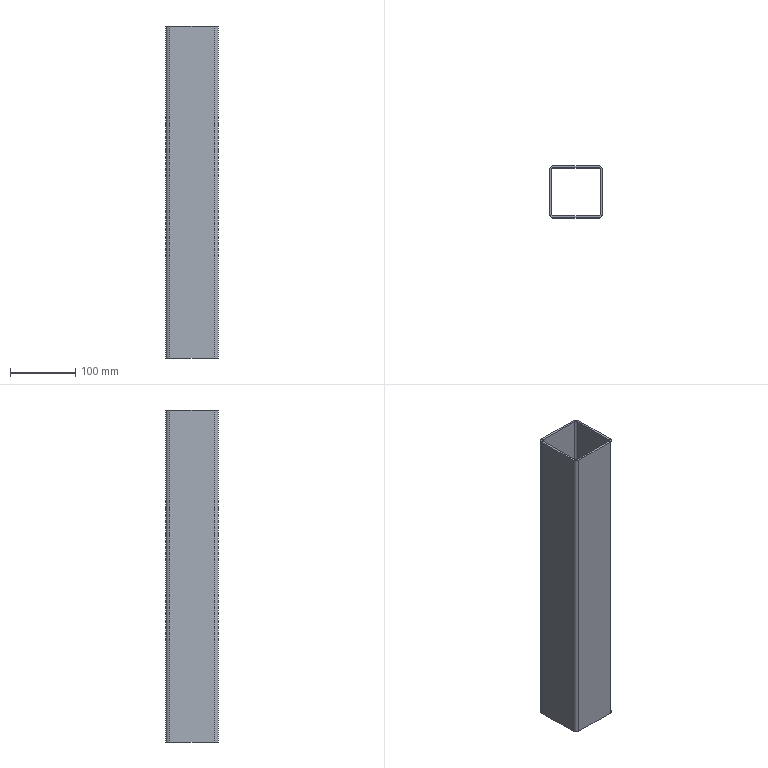Part | STEP file | Copy (1) of SN10_008_006-01_TUBO_QUADRADO | 1 solid | 18 faces | box 80 x 80 x 507.179 mm | volume 456879 mm3 | plane 10 | cylinder 8 | commonest cylinder face diameters 6 x4 12 x4
STEP:
#1=CARTESIAN_POINT('',(0.,0.,0.));
#2=DIRECTION('',(0.,0.,1.));
#3=DIRECTION('',(1.,0.,0.));
#4=AXIS2_PLACEMENT_3D('',#1,#2,#3);
#5=CARTESIAN_POINT('',(323.629,344.,-61.18));
#6=VERTEX_POINT('',#5);
#7=CARTESIAN_POINT('',(317.629,350.,-61.18));
#8=VERTEX_POINT('',#7);
#9=CARTESIAN_POINT('',(317.629,344.,-61.18));
#10=DIRECTION('',(0.,0.,1.));
#11=DIRECTION('',(1.,0.,0.));
#12=AXIS2_PLACEMENT_3D('',#9,#10,#11);
#13=CIRCLE('',#12,6.);
#14=CARTESIAN_POINT('',(361.047,350.,-61.18));
#15=DIRECTION('',(0.,0.,1.));
#16=DIRECTION('',(1.,0.,0.));
#17=AXIS2_PLACEMENT_3D('',#14,#15,#16);
#18=PLANE('',#17);
#19=CARTESIAN_POINT('',(-43.418,-6.));
#20=DIRECTION('',(1.,0.));
#21=AXIS2_PLACEMENT_2D('',#19,#20);
#22=CIRCLE('',#21,6.);
#23=(GEOMETRIC_REPRESENTATION_CONTEXT(2)PARAMETRIC_REPRESENTATION_CONTEXT()REPRESENTATION_CONTEXT('',''));
#24=DEFINITIONAL_REPRESENTATION('',(#22),#23);
#25=PCURVE('',#18,#24);
#26=CARTESIAN_POINT('',(317.629,344.,176.11));
#27=DIRECTION('',(0.,0.,1.));
#28=DIRECTION('',(1.,0.,0.));
#29=AXIS2_PLACEMENT_3D('',#26,#27,#28);
#30=CYLINDRICAL_SURFACE('',#29,6.);
#31=CARTESIAN_POINT('',(0.,-237.289));
#32=DIRECTION('',(1.,0.));
#33=VECTOR('',#32,1.);
#34=LINE('',#31,#33);
#35=(GEOMETRIC_REPRESENTATION_CONTEXT(2)PARAMETRIC_REPRESENTATION_CONTEXT()REPRESENTATION_CONTEXT('',''));
#36=DEFINITIONAL_REPRESENTATION('',(#34),#35);
#37=PCURVE('',#30,#36);
#38=SURFACE_CURVE('',#13,(#25,#37),.PCURVE_S1.);
#39=EDGE_CURVE('',#6,#8,#38,.T.);
#40=ORIENTED_EDGE('',*,*,#39,.F.);
#41=CARTESIAN_POINT('',(323.629,276.,-61.18));
#42=VERTEX_POINT('',#41);
#43=CARTESIAN_POINT('',(323.629,344.,-61.18));
#44=DIRECTION('',(0.,-1.,0.));
#45=VECTOR('',#44,1.);
#46=LINE('',#43,#45);
#47=CARTESIAN_POINT('',(-37.418,-6.));
#48=DIRECTION('',(0.,-1.));
#49=VECTOR('',#48,1.);
#50=LINE('',#47,#49);
#51=(GEOMETRIC_REPRESENTATION_CONTEXT(2)PARAMETRIC_REPRESENTATION_CONTEXT()REPRESENTATION_CONTEXT('',''));
#52=DEFINITIONAL_REPRESENTATION('',(#50),#51);
#53=PCURVE('',#18,#52);
#54=CARTESIAN_POINT('',(323.629,344.,-115.));
#55=DIRECTION('',(-1.,0.,0.));
#56=DIRECTION('',(0.,0.,1.));
#57=AXIS2_PLACEMENT_3D('',#54,#55,#56);
#58=PLANE('',#57);
#59=CARTESIAN_POINT('',(53.821,0.));
#60=DIRECTION('',(0.,-1.));
#61=VECTOR('',#60,1.);
#62=LINE('',#59,#61);
#63=(GEOMETRIC_REPRESENTATION_CONTEXT(2)PARAMETRIC_REPRESENTATION_CONTEXT()REPRESENTATION_CONTEXT('',''));
#64=DEFINITIONAL_REPRESENTATION('',(#62),#63);
#65=PCURVE('',#58,#64);
#66=SURFACE_CURVE('',#46,(#53,#65),.PCURVE_S1.);
#67=EDGE_CURVE('',#6,#42,#66,.T.);
#68=ORIENTED_EDGE('',*,*,#67,.T.);
#69=CARTESIAN_POINT('',(317.629,270.,-61.18));
#70=VERTEX_POINT('',#69);
#71=CARTESIAN_POINT('',(317.629,276.,-61.18));
#72=DIRECTION('',(0.,0.,1.));
#73=DIRECTION('',(1.,0.,0.));
#74=AXIS2_PLACEMENT_3D('',#71,#72,#73);
#75=CIRCLE('',#74,6.);
#76=CARTESIAN_POINT('',(-43.418,-74.));
#77=DIRECTION('',(1.,0.));
#78=AXIS2_PLACEMENT_2D('',#76,#77);
#79=CIRCLE('',#78,6.);
#80=(GEOMETRIC_REPRESENTATION_CONTEXT(2)PARAMETRIC_REPRESENTATION_CONTEXT()REPRESENTATION_CONTEXT('',''));
#81=DEFINITIONAL_REPRESENTATION('',(#79),#80);
#82=PCURVE('',#18,#81);
#83=CARTESIAN_POINT('',(317.629,276.,176.11));
#84=DIRECTION('',(0.,0.,1.));
#85=DIRECTION('',(0.,-1.,0.));
#86=AXIS2_PLACEMENT_3D('',#83,#84,#85);
#87=CYLINDRICAL_SURFACE('',#86,6.);
#88=CARTESIAN_POINT('',(-4.712,-237.289));
#89=DIRECTION('',(1.,0.));
#90=VECTOR('',#89,1.);
#91=LINE('',#88,#90);
#92=(GEOMETRIC_REPRESENTATION_CONTEXT(2)PARAMETRIC_REPRESENTATION_CONTEXT()REPRESENTATION_CONTEXT('',''));
#93=DEFINITIONAL_REPRESENTATION('',(#91),#92);
#94=PCURVE('',#87,#93);
#95=SURFACE_CURVE('',#75,(#82,#94),.PCURVE_S1.);
#96=EDGE_CURVE('',#70,#42,#95,.T.);
#97=ORIENTED_EDGE('',*,*,#96,.F.);
#98=CARTESIAN_POINT('',(249.629,270.,-61.18));
#99=VERTEX_POINT('',#98);
#100=CARTESIAN_POINT('',(317.629,270.,-61.18));
#101=DIRECTION('',(-1.,0.,0.));
#102=VECTOR('',#101,1.);
#103=LINE('',#100,#102);
#104=CARTESIAN_POINT('',(-43.418,-80.));
#105=DIRECTION('',(-1.,0.));
#106=VECTOR('',#105,1.);
#107=LINE('',#104,#106);
#108=(GEOMETRIC_REPRESENTATION_CONTEXT(2)PARAMETRIC_REPRESENTATION_CONTEXT()REPRESENTATION_CONTEXT('',''));
#109=DEFINITIONAL_REPRESENTATION('',(#107),#108);
#110=PCURVE('',#18,#109);
#111=CARTESIAN_POINT('',(317.629,270.,-115.));
#112=DIRECTION('',(0.,1.,0.));
#113=DIRECTION('',(0.,0.,1.));
#114=AXIS2_PLACEMENT_3D('',#111,#112,#113);
#115=PLANE('',#114);
#116=CARTESIAN_POINT('',(53.821,0.));
#117=DIRECTION('',(0.,-1.));
#118=VECTOR('',#117,1.);
#119=LINE('',#116,#118);
#120=(GEOMETRIC_REPRESENTATION_CONTEXT(2)PARAMETRIC_REPRESENTATION_CONTEXT()REPRESENTATION_CONTEXT('',''));
#121=DEFINITIONAL_REPRESENTATION('',(#119),#120);
#122=PCURVE('',#115,#121);
#123=SURFACE_CURVE('',#103,(#110,#122),.PCURVE_S1.);
#124=EDGE_CURVE('',#70,#99,#123,.T.);
#125=ORIENTED_EDGE('',*,*,#124,.T.);
#126=CARTESIAN_POINT('',(243.629,276.,-61.18));
#127=VERTEX_POINT('',#126);
#128=CARTESIAN_POINT('',(249.629,276.,-61.18));
#129=DIRECTION('',(0.,0.,1.));
#130=DIRECTION('',(1.,0.,0.));
#131=AXIS2_PLACEMENT_3D('',#128,#129,#130);
#132=CIRCLE('',#131,6.);
#133=CARTESIAN_POINT('',(-111.418,-74.));
#134=DIRECTION('',(1.,0.));
#135=AXIS2_PLACEMENT_2D('',#133,#134);
#136=CIRCLE('',#135,6.);
#137=(GEOMETRIC_REPRESENTATION_CONTEXT(2)PARAMETRIC_REPRESENTATION_CONTEXT()REPRESENTATION_CONTEXT('',''));
#138=DEFINITIONAL_REPRESENTATION('',(#136),#137);
#139=PCURVE('',#18,#138);
#140=CARTESIAN_POINT('',(249.629,276.,176.11));
#141=DIRECTION('',(0.,0.,1.));
#142=DIRECTION('',(-1.,0.,0.));
#143=AXIS2_PLACEMENT_3D('',#140,#141,#142);
#144=CYLINDRICAL_SURFACE('',#143,6.);
#145=CARTESIAN_POINT('',(-3.142,-237.289));
#146=DIRECTION('',(1.,0.));
#147=VECTOR('',#146,1.);
#148=LINE('',#145,#147);
#149=(GEOMETRIC_REPRESENTATION_CONTEXT(2)PARAMETRIC_REPRESENTATION_CONTEXT()REPRESENTATION_CONTEXT('',''));
#150=DEFINITIONAL_REPRESENTATION('',(#148),#149);
#151=PCURVE('',#144,#150);
#152=SURFACE_CURVE('',#132,(#139,#151),.PCURVE_S1.);
#153=EDGE_CURVE('',#127,#99,#152,.T.);
#154=ORIENTED_EDGE('',*,*,#153,.F.);
#155=CARTESIAN_POINT('',(243.629,344.,-61.18));
#156=VERTEX_POINT('',#155);
#157=CARTESIAN_POINT('',(243.629,276.,-61.18));
#158=DIRECTION('',(0.,1.,0.));
#159=VECTOR('',#158,1.);
#160=LINE('',#157,#159);
#161=CARTESIAN_POINT('',(-117.418,-74.));
#162=DIRECTION('',(0.,1.));
#163=VECTOR('',#162,1.);
#164=LINE('',#161,#163);
#165=(GEOMETRIC_REPRESENTATION_CONTEXT(2)PARAMETRIC_REPRESENTATION_CONTEXT()REPRESENTATION_CONTEXT('',''));
#166=DEFINITIONAL_REPRESENTATION('',(#164),#165);
#167=PCURVE('',#18,#166);
#168=CARTESIAN_POINT('',(243.629,276.,-115.));
#169=DIRECTION('',(1.,0.,0.));
#170=DIRECTION('',(0.,0.,-1.));
#171=AXIS2_PLACEMENT_3D('',#168,#169,#170);
#172=PLANE('',#171);
#173=CARTESIAN_POINT('',(-53.821,0.));
#174=DIRECTION('',(0.,1.));
#175=VECTOR('',#174,1.);
#176=LINE('',#173,#175);
#177=(GEOMETRIC_REPRESENTATION_CONTEXT(2)PARAMETRIC_REPRESENTATION_CONTEXT()REPRESENTATION_CONTEXT('',''));
#178=DEFINITIONAL_REPRESENTATION('',(#176),#177);
#179=PCURVE('',#172,#178);
#180=SURFACE_CURVE('',#160,(#167,#179),.PCURVE_S1.);
#181=EDGE_CURVE('',#127,#156,#180,.T.);
#182=ORIENTED_EDGE('',*,*,#181,.T.);
#183=CARTESIAN_POINT('',(249.629,350.,-61.18));
#184=VERTEX_POINT('',#183);
#185=CARTESIAN_POINT('',(249.629,344.,-61.18));
#186=DIRECTION('',(0.,0.,1.));
#187=DIRECTION('',(1.,0.,0.));
#188=AXIS2_PLACEMENT_3D('',#185,#186,#187);
#189=CIRCLE('',#188,6.);
#190=CARTESIAN_POINT('',(-111.418,-6.));
#191=DIRECTION('',(1.,0.));
#192=AXIS2_PLACEMENT_2D('',#190,#191);
#193=CIRCLE('',#192,6.);
#194=(GEOMETRIC_REPRESENTATION_CONTEXT(2)PARAMETRIC_REPRESENTATION_CONTEXT()REPRESENTATION_CONTEXT('',''));
#195=DEFINITIONAL_REPRESENTATION('',(#193),#194);
#196=PCURVE('',#18,#195);
#197=CARTESIAN_POINT('',(249.629,344.,176.11));
#198=DIRECTION('',(0.,0.,1.));
#199=DIRECTION('',(0.,1.,0.));
#200=AXIS2_PLACEMENT_3D('',#197,#198,#199);
#201=CYLINDRICAL_SURFACE('',#200,6.);
#202=CARTESIAN_POINT('',(-1.571,-237.289));
#203=DIRECTION('',(1.,0.));
#204=VECTOR('',#203,1.);
#205=LINE('',#202,#204);
#206=(GEOMETRIC_REPRESENTATION_CONTEXT(2)PARAMETRIC_REPRESENTATION_CONTEXT()REPRESENTATION_CONTEXT('',''));
#207=DEFINITIONAL_REPRESENTATION('',(#205),#206);
#208=PCURVE('',#201,#207);
#209=SURFACE_CURVE('',#189,(#196,#208),.PCURVE_S1.);
#210=EDGE_CURVE('',#184,#156,#209,.T.);
#211=ORIENTED_EDGE('',*,*,#210,.F.);
#212=CARTESIAN_POINT('',(317.629,350.,-61.18));
#213=DIRECTION('',(-1.,0.,0.));
#214=VECTOR('',#213,1.);
#215=LINE('',#212,#214);
#216=CARTESIAN_POINT('',(-43.418,0.));
#217=DIRECTION('',(-1.,0.));
#218=VECTOR('',#217,1.);
#219=LINE('',#216,#218);
#220=(GEOMETRIC_REPRESENTATION_CONTEXT(2)PARAMETRIC_REPRESENTATION_CONTEXT()REPRESENTATION_CONTEXT('',''));
#221=DEFINITIONAL_REPRESENTATION('',(#219),#220);
#222=PCURVE('',#18,#221);
#223=CARTESIAN_POINT('',(249.629,350.,-115.));
#224=DIRECTION('',(0.,-1.,0.));
#225=DIRECTION('',(0.,0.,-1.));
#226=AXIS2_PLACEMENT_3D('',#223,#224,#225);
#227=PLANE('',#226);
#228=CARTESIAN_POINT('',(-53.821,68.));
#229=DIRECTION('',(0.,-1.));
#230=VECTOR('',#229,1.);
#231=LINE('',#228,#230);
#232=(GEOMETRIC_REPRESENTATION_CONTEXT(2)PARAMETRIC_REPRESENTATION_CONTEXT()REPRESENTATION_CONTEXT('',''));
#233=DEFINITIONAL_REPRESENTATION('',(#231),#232);
#234=PCURVE('',#227,#233);
#235=SURFACE_CURVE('',#215,(#222,#234),.PCURVE_S1.);
#236=EDGE_CURVE('',#8,#184,#235,.T.);
#237=ORIENTED_EDGE('',*,*,#236,.F.);
#238=EDGE_LOOP('',(#40,#68,#97,#125,#154,#182,#211,#237));
#239=FACE_BOUND('',#238,.T.);
#240=CARTESIAN_POINT('',(249.629,347.,-61.18));
#241=VERTEX_POINT('',#240);
#242=CARTESIAN_POINT('',(246.629,344.,-61.18));
#243=VERTEX_POINT('',#242);
#244=CARTESIAN_POINT('',(249.629,344.,-61.18));
#245=DIRECTION('',(0.,0.,1.));
#246=DIRECTION('',(1.,0.,0.));
#247=AXIS2_PLACEMENT_3D('',#244,#245,#246);
#248=CIRCLE('',#247,3.);
#249=CARTESIAN_POINT('',(-111.418,-6.));
#250=DIRECTION('',(1.,0.));
#251=AXIS2_PLACEMENT_2D('',#249,#250);
#252=CIRCLE('',#251,3.);
#253=(GEOMETRIC_REPRESENTATION_CONTEXT(2)PARAMETRIC_REPRESENTATION_CONTEXT()REPRESENTATION_CONTEXT('',''));
#254=DEFINITIONAL_REPRESENTATION('',(#252),#253);
#255=PCURVE('',#18,#254);
#256=CARTESIAN_POINT('',(249.629,344.,176.11));
#257=DIRECTION('',(0.,0.,1.));
#258=DIRECTION('',(0.,1.,0.));
#259=AXIS2_PLACEMENT_3D('',#256,#257,#258);
#260=CYLINDRICAL_SURFACE('',#259,3.);
#261=CARTESIAN_POINT('',(-1.571,-237.289));
#262=DIRECTION('',(1.,0.));
#263=VECTOR('',#262,1.);
#264=LINE('',#261,#263);
#265=(GEOMETRIC_REPRESENTATION_CONTEXT(2)PARAMETRIC_REPRESENTATION_CONTEXT()REPRESENTATION_CONTEXT('',''));
#266=DEFINITIONAL_REPRESENTATION('',(#264),#265);
#267=PCURVE('',#260,#266);
#268=SURFACE_CURVE('',#248,(#255,#267),.PCURVE_S1.);
#269=EDGE_CURVE('',#241,#243,#268,.T.);
#270=ORIENTED_EDGE('',*,*,#269,.T.);
#271=CARTESIAN_POINT('',(246.629,276.,-61.18));
#272=VERTEX_POINT('',#271);
#273=CARTESIAN_POINT('',(246.629,276.,-61.18));
#274=DIRECTION('',(0.,1.,0.));
#275=VECTOR('',#274,1.);
#276=LINE('',#273,#275);
#277=CARTESIAN_POINT('',(-114.418,-74.));
#278=DIRECTION('',(0.,1.));
#279=VECTOR('',#278,1.);
#280=LINE('',#277,#279);
#281=(GEOMETRIC_REPRESENTATION_CONTEXT(2)PARAMETRIC_REPRESENTATION_CONTEXT()REPRESENTATION_CONTEXT('',''));
#282=DEFINITIONAL_REPRESENTATION('',(#280),#281);
#283=PCURVE('',#18,#282);
#284=CARTESIAN_POINT('',(246.629,276.,-115.));
#285=DIRECTION('',(1.,0.,0.));
#286=DIRECTION('',(0.,0.,-1.));
#287=AXIS2_PLACEMENT_3D('',#284,#285,#286);
#288=PLANE('',#287);
#289=CARTESIAN_POINT('',(-53.821,0.));
#290=DIRECTION('',(0.,1.));
#291=VECTOR('',#290,1.);
#292=LINE('',#289,#291);
#293=(GEOMETRIC_REPRESENTATION_CONTEXT(2)PARAMETRIC_REPRESENTATION_CONTEXT()REPRESENTATION_CONTEXT('',''));
#294=DEFINITIONAL_REPRESENTATION('',(#292),#293);
#295=PCURVE('',#288,#294);
#296=SURFACE_CURVE('',#276,(#283,#295),.PCURVE_S1.);
#297=EDGE_CURVE('',#272,#243,#296,.T.);
#298=ORIENTED_EDGE('',*,*,#297,.F.);
#299=CARTESIAN_POINT('',(249.629,273.,-61.18));
#300=VERTEX_POINT('',#299);
#301=CARTESIAN_POINT('',(249.629,276.,-61.18));
#302=DIRECTION('',(0.,0.,1.));
#303=DIRECTION('',(1.,0.,0.));
#304=AXIS2_PLACEMENT_3D('',#301,#302,#303);
#305=CIRCLE('',#304,3.);
#306=CARTESIAN_POINT('',(-111.418,-74.));
#307=DIRECTION('',(1.,0.));
#308=AXIS2_PLACEMENT_2D('',#306,#307);
#309=CIRCLE('',#308,3.);
#310=(GEOMETRIC_REPRESENTATION_CONTEXT(2)PARAMETRIC_REPRESENTATION_CONTEXT()REPRESENTATION_CONTEXT('',''));
#311=DEFINITIONAL_REPRESENTATION('',(#309),#310);
#312=PCURVE('',#18,#311);
#313=CARTESIAN_POINT('',(249.629,276.,176.11));
#314=DIRECTION('',(0.,0.,1.));
#315=DIRECTION('',(-1.,0.,0.));
#316=AXIS2_PLACEMENT_3D('',#313,#314,#315);
#317=CYLINDRICAL_SURFACE('',#316,3.);
#318=CARTESIAN_POINT('',(-3.142,-237.289));
#319=DIRECTION('',(1.,0.));
#320=VECTOR('',#319,1.);
#321=LINE('',#318,#320);
#322=(GEOMETRIC_REPRESENTATION_CONTEXT(2)PARAMETRIC_REPRESENTATION_CONTEXT()REPRESENTATION_CONTEXT('',''));
#323=DEFINITIONAL_REPRESENTATION('',(#321),#322);
#324=PCURVE('',#317,#323);
#325=SURFACE_CURVE('',#305,(#312,#324),.PCURVE_S1.);
#326=EDGE_CURVE('',#272,#300,#325,.T.);
#327=ORIENTED_EDGE('',*,*,#326,.T.);
#328=CARTESIAN_POINT('',(317.629,273.,-61.18));
#329=VERTEX_POINT('',#328);
#330=CARTESIAN_POINT('',(317.629,273.,-61.18));
#331=DIRECTION('',(-1.,0.,0.));
#332=VECTOR('',#331,1.);
#333=LINE('',#330,#332);
#334=CARTESIAN_POINT('',(-43.418,-77.));
#335=DIRECTION('',(-1.,0.));
#336=VECTOR('',#335,1.);
#337=LINE('',#334,#336);
#338=(GEOMETRIC_REPRESENTATION_CONTEXT(2)PARAMETRIC_REPRESENTATION_CONTEXT()REPRESENTATION_CONTEXT('',''));
#339=DEFINITIONAL_REPRESENTATION('',(#337),#338);
#340=PCURVE('',#18,#339);
#341=CARTESIAN_POINT('',(317.629,273.,-115.));
#342=DIRECTION('',(0.,1.,0.));
#343=DIRECTION('',(0.,0.,1.));
#344=AXIS2_PLACEMENT_3D('',#341,#342,#343);
#345=PLANE('',#344);
#346=CARTESIAN_POINT('',(53.821,0.));
#347=DIRECTION('',(0.,-1.));
#348=VECTOR('',#347,1.);
#349=LINE('',#346,#348);
#350=(GEOMETRIC_REPRESENTATION_CONTEXT(2)PARAMETRIC_REPRESENTATION_CONTEXT()REPRESENTATION_CONTEXT('',''));
#351=DEFINITIONAL_REPRESENTATION('',(#349),#350);
#352=PCURVE('',#345,#351);
#353=SURFACE_CURVE('',#333,(#340,#352),.PCURVE_S1.);
#354=EDGE_CURVE('',#329,#300,#353,.T.);
#355=ORIENTED_EDGE('',*,*,#354,.F.);
#356=CARTESIAN_POINT('',(320.629,276.,-61.18));
#357=VERTEX_POINT('',#356);
#358=CARTESIAN_POINT('',(317.629,276.,-61.18));
#359=DIRECTION('',(0.,0.,1.));
#360=DIRECTION('',(1.,0.,0.));
#361=AXIS2_PLACEMENT_3D('',#358,#359,#360);
#362=CIRCLE('',#361,3.);
#363=CARTESIAN_POINT('',(-43.418,-74.));
#364=DIRECTION('',(1.,0.));
#365=AXIS2_PLACEMENT_2D('',#363,#364);
#366=CIRCLE('',#365,3.);
#367=(GEOMETRIC_REPRESENTATION_CONTEXT(2)PARAMETRIC_REPRESENTATION_CONTEXT()REPRESENTATION_CONTEXT('',''));
#368=DEFINITIONAL_REPRESENTATION('',(#366),#367);
#369=PCURVE('',#18,#368);
#370=CARTESIAN_POINT('',(317.629,276.,176.11));
#371=DIRECTION('',(0.,0.,1.));
#372=DIRECTION('',(0.,-1.,0.));
#373=AXIS2_PLACEMENT_3D('',#370,#371,#372);
#374=CYLINDRICAL_SURFACE('',#373,3.);
#375=CARTESIAN_POINT('',(-4.712,-237.289));
#376=DIRECTION('',(1.,0.));
#377=VECTOR('',#376,1.);
#378=LINE('',#375,#377);
#379=(GEOMETRIC_REPRESENTATION_CONTEXT(2)PARAMETRIC_REPRESENTATION_CONTEXT()REPRESENTATION_CONTEXT('',''));
#380=DEFINITIONAL_REPRESENTATION('',(#378),#379);
#381=PCURVE('',#374,#380);
#382=SURFACE_CURVE('',#362,(#369,#381),.PCURVE_S1.);
#383=EDGE_CURVE('',#329,#357,#382,.T.);
#384=ORIENTED_EDGE('',*,*,#383,.T.);
#385=CARTESIAN_POINT('',(320.629,344.,-61.18));
#386=VERTEX_POINT('',#385);
#387=CARTESIAN_POINT('',(320.629,344.,-61.18));
#388=DIRECTION('',(0.,-1.,0.));
#389=VECTOR('',#388,1.);
#390=LINE('',#387,#389);
#391=CARTESIAN_POINT('',(-40.418,-6.));
#392=DIRECTION('',(0.,-1.));
#393=VECTOR('',#392,1.);
#394=LINE('',#391,#393);
#395=(GEOMETRIC_REPRESENTATION_CONTEXT(2)PARAMETRIC_REPRESENTATION_CONTEXT()REPRESENTATION_CONTEXT('',''));
#396=DEFINITIONAL_REPRESENTATION('',(#394),#395);
#397=PCURVE('',#18,#396);
#398=CARTESIAN_POINT('',(320.629,344.,-115.));
#399=DIRECTION('',(-1.,0.,0.));
#400=DIRECTION('',(0.,0.,1.));
#401=AXIS2_PLACEMENT_3D('',#398,#399,#400);
#402=PLANE('',#401);
#403=CARTESIAN_POINT('',(53.821,0.));
#404=DIRECTION('',(0.,-1.));
#405=VECTOR('',#404,1.);
#406=LINE('',#403,#405);
#407=(GEOMETRIC_REPRESENTATION_CONTEXT(2)PARAMETRIC_REPRESENTATION_CONTEXT()REPRESENTATION_CONTEXT('',''));
#408=DEFINITIONAL_REPRESENTATION('',(#406),#407);
#409=PCURVE('',#402,#408);
#410=SURFACE_CURVE('',#390,(#397,#409),.PCURVE_S1.);
#411=EDGE_CURVE('',#386,#357,#410,.T.);
#412=ORIENTED_EDGE('',*,*,#411,.F.);
#413=CARTESIAN_POINT('',(317.629,347.,-61.18));
#414=VERTEX_POINT('',#413);
#415=CARTESIAN_POINT('',(317.629,344.,-61.18));
#416=DIRECTION('',(0.,0.,1.));
#417=DIRECTION('',(1.,0.,0.));
#418=AXIS2_PLACEMENT_3D('',#415,#416,#417);
#419=CIRCLE('',#418,3.);
#420=CARTESIAN_POINT('',(-43.418,-6.));
#421=DIRECTION('',(1.,0.));
#422=AXIS2_PLACEMENT_2D('',#420,#421);
#423=CIRCLE('',#422,3.);
#424=(GEOMETRIC_REPRESENTATION_CONTEXT(2)PARAMETRIC_REPRESENTATION_CONTEXT()REPRESENTATION_CONTEXT('',''));
#425=DEFINITIONAL_REPRESENTATION('',(#423),#424);
#426=PCURVE('',#18,#425);
#427=CARTESIAN_POINT('',(317.629,344.,176.11));
#428=DIRECTION('',(0.,0.,1.));
#429=DIRECTION('',(1.,0.,0.));
#430=AXIS2_PLACEMENT_3D('',#427,#428,#429);
#431=CYLINDRICAL_SURFACE('',#430,3.);
#432=CARTESIAN_POINT('',(0.,-237.289));
#433=DIRECTION('',(1.,0.));
#434=VECTOR('',#433,1.);
#435=LINE('',#432,#434);
#436=(GEOMETRIC_REPRESENTATION_CONTEXT(2)PARAMETRIC_REPRESENTATION_CONTEXT()REPRESENTATION_CONTEXT('',''));
#437=DEFINITIONAL_REPRESENTATION('',(#435),#436);
#438=PCURVE('',#431,#437);
#439=SURFACE_CURVE('',#419,(#426,#438),.PCURVE_S1.);
#440=EDGE_CURVE('',#386,#414,#439,.T.);
#441=ORIENTED_EDGE('',*,*,#440,.T.);
#442=CARTESIAN_POINT('',(249.629,347.,-61.18));
#443=DIRECTION('',(1.,0.,0.));
#444=VECTOR('',#443,1.);
#445=LINE('',#442,#444);
#446=CARTESIAN_POINT('',(-111.418,-3.));
#447=DIRECTION('',(1.,0.));
#448=VECTOR('',#447,1.);
#449=LINE('',#446,#448);
#450=(GEOMETRIC_REPRESENTATION_CONTEXT(2)PARAMETRIC_REPRESENTATION_CONTEXT()REPRESENTATION_CONTEXT('',''));
#451=DEFINITIONAL_REPRESENTATION('',(#449),#450);
#452=PCURVE('',#18,#451);
#453=CARTESIAN_POINT('',(249.629,347.,-115.));
#454=DIRECTION('',(0.,-1.,0.));
#455=DIRECTION('',(0.,0.,-1.));
#456=AXIS2_PLACEMENT_3D('',#453,#454,#455);
#457=PLANE('',#456);
#458=CARTESIAN_POINT('',(-53.821,0.));
#459=DIRECTION('',(0.,1.));
#460=VECTOR('',#459,1.);
#461=LINE('',#458,#460);
#462=(GEOMETRIC_REPRESENTATION_CONTEXT(2)PARAMETRIC_REPRESENTATION_CONTEXT()REPRESENTATION_CONTEXT('',''));
#463=DEFINITIONAL_REPRESENTATION('',(#461),#462);
#464=PCURVE('',#457,#463);
#465=SURFACE_CURVE('',#445,(#452,#464),.PCURVE_S1.);
#466=EDGE_CURVE('',#241,#414,#465,.T.);
#467=ORIENTED_EDGE('',*,*,#466,.F.);
#468=EDGE_LOOP('',(#270,#298,#327,#355,#384,#412,#441,#467));
#469=FACE_BOUND('',#468,.T.);
#470=ADVANCED_FACE('',(#239,#469),#18,.F.);
#471=ORIENTED_EDGE('',*,*,#236,.T.);
#472=CARTESIAN_POINT('',(249.629,350.,446.));
#473=VERTEX_POINT('',#472);
#474=CARTESIAN_POINT('',(249.629,350.,446.));
#475=DIRECTION('',(0.,0.,-1.));
#476=VECTOR('',#475,1.);
#477=LINE('',#474,#476);
#478=CARTESIAN_POINT('',(-561.,0.));
#479=DIRECTION('',(1.,0.));
#480=VECTOR('',#479,1.);
#481=LINE('',#478,#480);
#482=(GEOMETRIC_REPRESENTATION_CONTEXT(2)PARAMETRIC_REPRESENTATION_CONTEXT()REPRESENTATION_CONTEXT('',''));
#483=DEFINITIONAL_REPRESENTATION('',(#481),#482);
#484=PCURVE('',#227,#483);
#485=CARTESIAN_POINT('',(0.,269.89));
#486=DIRECTION('',(0.,-1.));
#487=VECTOR('',#486,1.);
#488=LINE('',#485,#487);
#489=(GEOMETRIC_REPRESENTATION_CONTEXT(2)PARAMETRIC_REPRESENTATION_CONTEXT()REPRESENTATION_CONTEXT('',''));
#490=DEFINITIONAL_REPRESENTATION('',(#488),#489);
#491=PCURVE('',#201,#490);
#492=SURFACE_CURVE('',#477,(#484,#491),.PCURVE_S1.);
#493=EDGE_CURVE('',#473,#184,#492,.T.);
#494=ORIENTED_EDGE('',*,*,#493,.F.);
#495=CARTESIAN_POINT('',(317.629,350.,446.));
#496=VERTEX_POINT('',#495);
#497=CARTESIAN_POINT('',(249.629,350.,446.));
#498=DIRECTION('',(1.,0.,0.));
#499=VECTOR('',#498,1.);
#500=LINE('',#497,#499);
#501=CARTESIAN_POINT('',(-561.,0.));
#502=DIRECTION('',(0.,1.));
#503=VECTOR('',#502,1.);
#504=LINE('',#501,#503);
#505=(GEOMETRIC_REPRESENTATION_CONTEXT(2)PARAMETRIC_REPRESENTATION_CONTEXT()REPRESENTATION_CONTEXT('',''));
#506=DEFINITIONAL_REPRESENTATION('',(#504),#505);
#507=PCURVE('',#227,#506);
#508=CARTESIAN_POINT('',(323.629,250.,446.));
#509=DIRECTION('',(0.,0.,-1.));
#510=DIRECTION('',(-1.,0.,0.));
#511=AXIS2_PLACEMENT_3D('',#508,#509,#510);
#512=PLANE('',#511);
#513=CARTESIAN_POINT('',(74.,100.));
#514=DIRECTION('',(-1.,0.));
#515=VECTOR('',#514,1.);
#516=LINE('',#513,#515);
#517=(GEOMETRIC_REPRESENTATION_CONTEXT(2)PARAMETRIC_REPRESENTATION_CONTEXT()REPRESENTATION_CONTEXT('',''));
#518=DEFINITIONAL_REPRESENTATION('',(#516),#517);
#519=PCURVE('',#512,#518);
#520=SURFACE_CURVE('',#500,(#507,#519),.PCURVE_S1.);
#521=EDGE_CURVE('',#473,#496,#520,.T.);
#522=ORIENTED_EDGE('',*,*,#521,.T.);
#523=CARTESIAN_POINT('',(317.629,350.,446.));
#524=DIRECTION('',(0.,0.,-1.));
#525=VECTOR('',#524,1.);
#526=LINE('',#523,#525);
#527=CARTESIAN_POINT('',(-561.,68.));
#528=DIRECTION('',(1.,0.));
#529=VECTOR('',#528,1.);
#530=LINE('',#527,#529);
#531=(GEOMETRIC_REPRESENTATION_CONTEXT(2)PARAMETRIC_REPRESENTATION_CONTEXT()REPRESENTATION_CONTEXT('',''));
#532=DEFINITIONAL_REPRESENTATION('',(#530),#531);
#533=PCURVE('',#227,#532);
#534=CARTESIAN_POINT('',(1.571,269.89));
#535=DIRECTION('',(0.,-1.));
#536=VECTOR('',#535,1.);
#537=LINE('',#534,#536);
#538=(GEOMETRIC_REPRESENTATION_CONTEXT(2)PARAMETRIC_REPRESENTATION_CONTEXT()REPRESENTATION_CONTEXT('',''));
#539=DEFINITIONAL_REPRESENTATION('',(#537),#538);
#540=PCURVE('',#30,#539);
#541=SURFACE_CURVE('',#526,(#533,#540),.PCURVE_S1.);
#542=EDGE_CURVE('',#496,#8,#541,.T.);
#543=ORIENTED_EDGE('',*,*,#542,.T.);
#544=EDGE_LOOP('',(#471,#494,#522,#543));
#545=FACE_BOUND('',#544,.T.);
#546=ADVANCED_FACE('',(#545),#227,.F.);
#547=ORIENTED_EDGE('',*,*,#181,.F.);
#548=CARTESIAN_POINT('',(243.629,276.,446.));
#549=VERTEX_POINT('',#548);
#550=CARTESIAN_POINT('',(243.629,276.,446.));
#551=DIRECTION('',(0.,0.,-1.));
#552=VECTOR('',#551,1.);
#553=LINE('',#550,#552);
#554=CARTESIAN_POINT('',(-561.,0.));
#555=DIRECTION('',(1.,0.));
#556=VECTOR('',#555,1.);
#557=LINE('',#554,#556);
#558=(GEOMETRIC_REPRESENTATION_CONTEXT(2)PARAMETRIC_REPRESENTATION_CONTEXT()REPRESENTATION_CONTEXT('',''));
#559=DEFINITIONAL_REPRESENTATION('',(#557),#558);
#560=PCURVE('',#172,#559);
#561=CARTESIAN_POINT('',(0.,269.89));
#562=DIRECTION('',(0.,-1.));
#563=VECTOR('',#562,1.);
#564=LINE('',#561,#563);
#565=(GEOMETRIC_REPRESENTATION_CONTEXT(2)PARAMETRIC_REPRESENTATION_CONTEXT()REPRESENTATION_CONTEXT('',''));
#566=DEFINITIONAL_REPRESENTATION('',(#564),#565);
#567=PCURVE('',#144,#566);
#568=SURFACE_CURVE('',#553,(#560,#567),.PCURVE_S1.);
#569=EDGE_CURVE('',#549,#127,#568,.T.);
#570=ORIENTED_EDGE('',*,*,#569,.F.);
#571=CARTESIAN_POINT('',(243.629,344.,446.));
#572=VERTEX_POINT('',#571);
#573=CARTESIAN_POINT('',(243.629,276.,446.));
#574=DIRECTION('',(0.,1.,0.));
#575=VECTOR('',#574,1.);
#576=LINE('',#573,#575);
#577=CARTESIAN_POINT('',(-561.,0.));
#578=DIRECTION('',(0.,1.));
#579=VECTOR('',#578,1.);
#580=LINE('',#577,#579);
#581=(GEOMETRIC_REPRESENTATION_CONTEXT(2)PARAMETRIC_REPRESENTATION_CONTEXT()REPRESENTATION_CONTEXT('',''));
#582=DEFINITIONAL_REPRESENTATION('',(#580),#581);
#583=PCURVE('',#172,#582);
#584=CARTESIAN_POINT('',(80.,26.));
#585=DIRECTION('',(0.,1.));
#586=VECTOR('',#585,1.);
#587=LINE('',#584,#586);
#588=(GEOMETRIC_REPRESENTATION_CONTEXT(2)PARAMETRIC_REPRESENTATION_CONTEXT()REPRESENTATION_CONTEXT('',''));
#589=DEFINITIONAL_REPRESENTATION('',(#587),#588);
#590=PCURVE('',#512,#589);
#591=SURFACE_CURVE('',#576,(#583,#590),.PCURVE_S1.);
#592=EDGE_CURVE('',#549,#572,#591,.T.);
#593=ORIENTED_EDGE('',*,*,#592,.T.);
#594=CARTESIAN_POINT('',(243.629,344.,446.));
#595=DIRECTION('',(0.,0.,-1.));
#596=VECTOR('',#595,1.);
#597=LINE('',#594,#596);
#598=CARTESIAN_POINT('',(-561.,68.));
#599=DIRECTION('',(1.,0.));
#600=VECTOR('',#599,1.);
#601=LINE('',#598,#600);
#602=(GEOMETRIC_REPRESENTATION_CONTEXT(2)PARAMETRIC_REPRESENTATION_CONTEXT()REPRESENTATION_CONTEXT('',''));
#603=DEFINITIONAL_REPRESENTATION('',(#601),#602);
#604=PCURVE('',#172,#603);
#605=CARTESIAN_POINT('',(1.571,269.89));
#606=DIRECTION('',(0.,-1.));
#607=VECTOR('',#606,1.);
#608=LINE('',#605,#607);
#609=(GEOMETRIC_REPRESENTATION_CONTEXT(2)PARAMETRIC_REPRESENTATION_CONTEXT()REPRESENTATION_CONTEXT('',''));
#610=DEFINITIONAL_REPRESENTATION('',(#608),#609);
#611=PCURVE('',#201,#610);
#612=SURFACE_CURVE('',#597,(#604,#611),.PCURVE_S1.);
#613=EDGE_CURVE('',#572,#156,#612,.T.);
#614=ORIENTED_EDGE('',*,*,#613,.T.);
#615=EDGE_LOOP('',(#547,#570,#593,#614));
#616=FACE_BOUND('',#615,.T.);
#617=ADVANCED_FACE('',(#616),#172,.F.);
#618=ORIENTED_EDGE('',*,*,#124,.F.);
#619=CARTESIAN_POINT('',(317.629,270.,446.));
#620=VERTEX_POINT('',#619);
#621=CARTESIAN_POINT('',(317.629,270.,446.));
#622=DIRECTION('',(0.,0.,-1.));
#623=VECTOR('',#622,1.);
#624=LINE('',#621,#623);
#625=CARTESIAN_POINT('',(561.,0.));
#626=DIRECTION('',(-1.,0.));
#627=VECTOR('',#626,1.);
#628=LINE('',#625,#627);
#629=(GEOMETRIC_REPRESENTATION_CONTEXT(2)PARAMETRIC_REPRESENTATION_CONTEXT()REPRESENTATION_CONTEXT('',''));
#630=DEFINITIONAL_REPRESENTATION('',(#628),#629);
#631=PCURVE('',#115,#630);
#632=CARTESIAN_POINT('',(0.,269.89));
#633=DIRECTION('',(0.,-1.));
#634=VECTOR('',#633,1.);
#635=LINE('',#632,#634);
#636=(GEOMETRIC_REPRESENTATION_CONTEXT(2)PARAMETRIC_REPRESENTATION_CONTEXT()REPRESENTATION_CONTEXT('',''));
#637=DEFINITIONAL_REPRESENTATION('',(#635),#636);
#638=PCURVE('',#87,#637);
#639=SURFACE_CURVE('',#624,(#631,#638),.PCURVE_S1.);
#640=EDGE_CURVE('',#620,#70,#639,.T.);
#641=ORIENTED_EDGE('',*,*,#640,.F.);
#642=CARTESIAN_POINT('',(249.629,270.,446.));
#643=VERTEX_POINT('',#642);
#644=CARTESIAN_POINT('',(317.629,270.,446.));
#645=DIRECTION('',(-1.,0.,0.));
#646=VECTOR('',#645,1.);
#647=LINE('',#644,#646);
#648=CARTESIAN_POINT('',(561.,0.));
#649=DIRECTION('',(0.,-1.));
#650=VECTOR('',#649,1.);
#651=LINE('',#648,#650);
#652=(GEOMETRIC_REPRESENTATION_CONTEXT(2)PARAMETRIC_REPRESENTATION_CONTEXT()REPRESENTATION_CONTEXT('',''));
#653=DEFINITIONAL_REPRESENTATION('',(#651),#652);
#654=PCURVE('',#115,#653);
#655=CARTESIAN_POINT('',(6.,20.));
#656=DIRECTION('',(1.,0.));
#657=VECTOR('',#656,1.);
#658=LINE('',#655,#657);
#659=(GEOMETRIC_REPRESENTATION_CONTEXT(2)PARAMETRIC_REPRESENTATION_CONTEXT()REPRESENTATION_CONTEXT('',''));
#660=DEFINITIONAL_REPRESENTATION('',(#658),#659);
#661=PCURVE('',#512,#660);
#662=SURFACE_CURVE('',#647,(#654,#661),.PCURVE_S1.);
#663=EDGE_CURVE('',#620,#643,#662,.T.);
#664=ORIENTED_EDGE('',*,*,#663,.T.);
#665=CARTESIAN_POINT('',(249.629,270.,446.));
#666=DIRECTION('',(0.,0.,-1.));
#667=VECTOR('',#666,1.);
#668=LINE('',#665,#667);
#669=CARTESIAN_POINT('',(561.,-68.));
#670=DIRECTION('',(-1.,0.));
#671=VECTOR('',#670,1.);
#672=LINE('',#669,#671);
#673=(GEOMETRIC_REPRESENTATION_CONTEXT(2)PARAMETRIC_REPRESENTATION_CONTEXT()REPRESENTATION_CONTEXT('',''));
#674=DEFINITIONAL_REPRESENTATION('',(#672),#673);
#675=PCURVE('',#115,#674);
#676=CARTESIAN_POINT('',(1.571,269.89));
#677=DIRECTION('',(0.,-1.));
#678=VECTOR('',#677,1.);
#679=LINE('',#676,#678);
#680=(GEOMETRIC_REPRESENTATION_CONTEXT(2)PARAMETRIC_REPRESENTATION_CONTEXT()REPRESENTATION_CONTEXT('',''));
#681=DEFINITIONAL_REPRESENTATION('',(#679),#680);
#682=PCURVE('',#144,#681);
#683=SURFACE_CURVE('',#668,(#675,#682),.PCURVE_S1.);
#684=EDGE_CURVE('',#643,#99,#683,.T.);
#685=ORIENTED_EDGE('',*,*,#684,.T.);
#686=EDGE_LOOP('',(#618,#641,#664,#685));
#687=FACE_BOUND('',#686,.T.);
#688=ADVANCED_FACE('',(#687),#115,.F.);
#689=ORIENTED_EDGE('',*,*,#67,.F.);
#690=CARTESIAN_POINT('',(323.629,344.,446.));
#691=VERTEX_POINT('',#690);
#692=CARTESIAN_POINT('',(323.629,344.,446.));
#693=DIRECTION('',(0.,0.,-1.));
#694=VECTOR('',#693,1.);
#695=LINE('',#692,#694);
#696=CARTESIAN_POINT('',(561.,0.));
#697=DIRECTION('',(-1.,0.));
#698=VECTOR('',#697,1.);
#699=LINE('',#696,#698);
#700=(GEOMETRIC_REPRESENTATION_CONTEXT(2)PARAMETRIC_REPRESENTATION_CONTEXT()REPRESENTATION_CONTEXT('',''));
#701=DEFINITIONAL_REPRESENTATION('',(#699),#700);
#702=PCURVE('',#58,#701);
#703=CARTESIAN_POINT('',(0.,269.89));
#704=DIRECTION('',(0.,-1.));
#705=VECTOR('',#704,1.);
#706=LINE('',#703,#705);
#707=(GEOMETRIC_REPRESENTATION_CONTEXT(2)PARAMETRIC_REPRESENTATION_CONTEXT()REPRESENTATION_CONTEXT('',''));
#708=DEFINITIONAL_REPRESENTATION('',(#706),#707);
#709=PCURVE('',#30,#708);
#710=SURFACE_CURVE('',#695,(#702,#709),.PCURVE_S1.);
#711=EDGE_CURVE('',#691,#6,#710,.T.);
#712=ORIENTED_EDGE('',*,*,#711,.F.);
#713=CARTESIAN_POINT('',(323.629,276.,446.));
#714=VERTEX_POINT('',#713);
#715=CARTESIAN_POINT('',(323.629,344.,446.));
#716=DIRECTION('',(0.,-1.,0.));
#717=VECTOR('',#716,1.);
#718=LINE('',#715,#717);
#719=CARTESIAN_POINT('',(561.,0.));
#720=DIRECTION('',(0.,-1.));
#721=VECTOR('',#720,1.);
#722=LINE('',#719,#721);
#723=(GEOMETRIC_REPRESENTATION_CONTEXT(2)PARAMETRIC_REPRESENTATION_CONTEXT()REPRESENTATION_CONTEXT('',''));
#724=DEFINITIONAL_REPRESENTATION('',(#722),#723);
#725=PCURVE('',#58,#724);
#726=CARTESIAN_POINT('',(0.,94.));
#727=DIRECTION('',(0.,-1.));
#728=VECTOR('',#727,1.);
#729=LINE('',#726,#728);
#730=(GEOMETRIC_REPRESENTATION_CONTEXT(2)PARAMETRIC_REPRESENTATION_CONTEXT()REPRESENTATION_CONTEXT('',''));
#731=DEFINITIONAL_REPRESENTATION('',(#729),#730);
#732=PCURVE('',#512,#731);
#733=SURFACE_CURVE('',#718,(#725,#732),.PCURVE_S1.);
#734=EDGE_CURVE('',#691,#714,#733,.T.);
#735=ORIENTED_EDGE('',*,*,#734,.T.);
#736=CARTESIAN_POINT('',(323.629,276.,446.));
#737=DIRECTION('',(0.,0.,-1.));
#738=VECTOR('',#737,1.);
#739=LINE('',#736,#738);
#740=CARTESIAN_POINT('',(561.,-68.));
#741=DIRECTION('',(-1.,0.));
#742=VECTOR('',#741,1.);
#743=LINE('',#740,#742);
#744=(GEOMETRIC_REPRESENTATION_CONTEXT(2)PARAMETRIC_REPRESENTATION_CONTEXT()REPRESENTATION_CONTEXT('',''));
#745=DEFINITIONAL_REPRESENTATION('',(#743),#744);
#746=PCURVE('',#58,#745);
#747=CARTESIAN_POINT('',(1.571,269.89));
#748=DIRECTION('',(0.,-1.));
#749=VECTOR('',#748,1.);
#750=LINE('',#747,#749);
#751=(GEOMETRIC_REPRESENTATION_CONTEXT(2)PARAMETRIC_REPRESENTATION_CONTEXT()REPRESENTATION_CONTEXT('',''));
#752=DEFINITIONAL_REPRESENTATION('',(#750),#751);
#753=PCURVE('',#87,#752);
#754=SURFACE_CURVE('',#739,(#746,#753),.PCURVE_S1.);
#755=EDGE_CURVE('',#714,#42,#754,.T.);
#756=ORIENTED_EDGE('',*,*,#755,.T.);
#757=EDGE_LOOP('',(#689,#712,#735,#756));
#758=FACE_BOUND('',#757,.T.);
#759=ADVANCED_FACE('',(#758),#58,.F.);
#760=CARTESIAN_POINT('',(317.629,347.,446.));
#761=VERTEX_POINT('',#760);
#762=CARTESIAN_POINT('',(317.629,347.,-61.18));
#763=DIRECTION('',(0.,0.,1.));
#764=VECTOR('',#763,1.);
#765=LINE('',#762,#764);
#766=CARTESIAN_POINT('',(1.571,-237.289));
#767=DIRECTION('',(0.,1.));
#768=VECTOR('',#767,1.);
#769=LINE('',#766,#768);
#770=(GEOMETRIC_REPRESENTATION_CONTEXT(2)PARAMETRIC_REPRESENTATION_CONTEXT()REPRESENTATION_CONTEXT('',''));
#771=DEFINITIONAL_REPRESENTATION('',(#769),#770);
#772=PCURVE('',#431,#771);
#773=CARTESIAN_POINT('',(-53.821,68.));
#774=DIRECTION('',(-1.,0.));
#775=VECTOR('',#774,1.);
#776=LINE('',#773,#775);
#777=(GEOMETRIC_REPRESENTATION_CONTEXT(2)PARAMETRIC_REPRESENTATION_CONTEXT()REPRESENTATION_CONTEXT('',''));
#778=DEFINITIONAL_REPRESENTATION('',(#776),#777);
#779=PCURVE('',#457,#778);
#780=SURFACE_CURVE('',#765,(#772,#779),.PCURVE_S1.);
#781=EDGE_CURVE('',#414,#761,#780,.T.);
#782=ORIENTED_EDGE('',*,*,#781,.T.);
#783=CARTESIAN_POINT('',(320.629,344.,446.));
#784=VERTEX_POINT('',#783);
#785=CARTESIAN_POINT('',(317.629,344.,446.));
#786=DIRECTION('',(0.,0.,1.));
#787=DIRECTION('',(1.,0.,0.));
#788=AXIS2_PLACEMENT_3D('',#785,#786,#787);
#789=CIRCLE('',#788,3.);
#790=CARTESIAN_POINT('',(0.,269.89));
#791=DIRECTION('',(1.,0.));
#792=VECTOR('',#791,1.);
#793=LINE('',#790,#792);
#794=(GEOMETRIC_REPRESENTATION_CONTEXT(2)PARAMETRIC_REPRESENTATION_CONTEXT()REPRESENTATION_CONTEXT('',''));
#795=DEFINITIONAL_REPRESENTATION('',(#793),#794);
#796=PCURVE('',#431,#795);
#797=CARTESIAN_POINT('',(3.,94.));
#798=CARTESIAN_POINT('',(3.,99.196));
#799=CARTESIAN_POINT('',(7.5,96.598));
#800=CARTESIAN_POINT('',(12.,94.));
#801=CARTESIAN_POINT('',(7.5,91.402));
#802=CARTESIAN_POINT('',(3.,88.804));
#803=CARTESIAN_POINT('',(3.,94.));
#804=(BOUNDED_CURVE()B_SPLINE_CURVE(2,(#797,#798,#799,#800,#801,#802,#803),.UNSPECIFIED.,.T.,.F.)B_SPLINE_CURVE_WITH_KNOTS((1,2,2,2,2,1),(-2.094,0.,2.094,4.189,6.283,8.378),.UNSPECIFIED.)CURVE()GEOMETRIC_REPRESENTATION_ITEM()RATIONAL_B_SPLINE_CURVE((1.,0.5,1.,0.5,1.,0.5,1.))REPRESENTATION_ITEM(''));
#805=(GEOMETRIC_REPRESENTATION_CONTEXT(2)PARAMETRIC_REPRESENTATION_CONTEXT()REPRESENTATION_CONTEXT('',''));
#806=DEFINITIONAL_REPRESENTATION('',(#804),#805);
#807=PCURVE('',#512,#806);
#808=SURFACE_CURVE('',#789,(#796,#807),.PCURVE_S1.);
#809=EDGE_CURVE('',#784,#761,#808,.T.);
#810=ORIENTED_EDGE('',*,*,#809,.F.);
#811=CARTESIAN_POINT('',(320.629,344.,-61.18));
#812=DIRECTION('',(0.,0.,1.));
#813=VECTOR('',#812,1.);
#814=LINE('',#811,#813);
#815=CARTESIAN_POINT('',(0.,-237.289));
#816=DIRECTION('',(0.,1.));
#817=VECTOR('',#816,1.);
#818=LINE('',#815,#817);
#819=(GEOMETRIC_REPRESENTATION_CONTEXT(2)PARAMETRIC_REPRESENTATION_CONTEXT()REPRESENTATION_CONTEXT('',''));
#820=DEFINITIONAL_REPRESENTATION('',(#818),#819);
#821=PCURVE('',#431,#820);
#822=CARTESIAN_POINT('',(53.821,0.));
#823=DIRECTION('',(1.,0.));
#824=VECTOR('',#823,1.);
#825=LINE('',#822,#824);
#826=(GEOMETRIC_REPRESENTATION_CONTEXT(2)PARAMETRIC_REPRESENTATION_CONTEXT()REPRESENTATION_CONTEXT('',''));
#827=DEFINITIONAL_REPRESENTATION('',(#825),#826);
#828=PCURVE('',#402,#827);
#829=SURFACE_CURVE('',#814,(#821,#828),.PCURVE_S1.);
#830=EDGE_CURVE('',#386,#784,#829,.T.);
#831=ORIENTED_EDGE('',*,*,#830,.F.);
#832=ORIENTED_EDGE('',*,*,#440,.T.);
#833=EDGE_LOOP('',(#782,#810,#831,#832));
#834=FACE_BOUND('',#833,.F.);
#835=ADVANCED_FACE('',(#834),#431,.F.);
#836=CARTESIAN_POINT('',(320.629,276.,446.));
#837=VERTEX_POINT('',#836);
#838=CARTESIAN_POINT('',(320.629,276.,-61.18));
#839=DIRECTION('',(0.,0.,1.));
#840=VECTOR('',#839,1.);
#841=LINE('',#838,#840);
#842=CARTESIAN_POINT('',(1.571,-237.289));
#843=DIRECTION('',(0.,1.));
#844=VECTOR('',#843,1.);
#845=LINE('',#842,#844);
#846=(GEOMETRIC_REPRESENTATION_CONTEXT(2)PARAMETRIC_REPRESENTATION_CONTEXT()REPRESENTATION_CONTEXT('',''));
#847=DEFINITIONAL_REPRESENTATION('',(#845),#846);
#848=PCURVE('',#374,#847);
#849=CARTESIAN_POINT('',(53.821,-68.));
#850=DIRECTION('',(1.,0.));
#851=VECTOR('',#850,1.);
#852=LINE('',#849,#851);
#853=(GEOMETRIC_REPRESENTATION_CONTEXT(2)PARAMETRIC_REPRESENTATION_CONTEXT()REPRESENTATION_CONTEXT('',''));
#854=DEFINITIONAL_REPRESENTATION('',(#852),#853);
#855=PCURVE('',#402,#854);
#856=SURFACE_CURVE('',#841,(#848,#855),.PCURVE_S1.);
#857=EDGE_CURVE('',#357,#837,#856,.T.);
#858=ORIENTED_EDGE('',*,*,#857,.T.);
#859=CARTESIAN_POINT('',(317.629,273.,446.));
#860=VERTEX_POINT('',#859);
#861=CARTESIAN_POINT('',(317.629,276.,446.));
#862=DIRECTION('',(0.,0.,1.));
#863=DIRECTION('',(1.,0.,0.));
#864=AXIS2_PLACEMENT_3D('',#861,#862,#863);
#865=CIRCLE('',#864,3.);
#866=CARTESIAN_POINT('',(-4.712,269.89));
#867=DIRECTION('',(1.,0.));
#868=VECTOR('',#867,1.);
#869=LINE('',#866,#868);
#870=(GEOMETRIC_REPRESENTATION_CONTEXT(2)PARAMETRIC_REPRESENTATION_CONTEXT()REPRESENTATION_CONTEXT('',''));
#871=DEFINITIONAL_REPRESENTATION('',(#869),#870);
#872=PCURVE('',#374,#871);
#873=CARTESIAN_POINT('',(3.,26.));
#874=CARTESIAN_POINT('',(3.,31.196));
#875=CARTESIAN_POINT('',(7.5,28.598));
#876=CARTESIAN_POINT('',(12.,26.));
#877=CARTESIAN_POINT('',(7.5,23.402));
#878=CARTESIAN_POINT('',(3.,20.804));
#879=CARTESIAN_POINT('',(3.,26.));
#880=(BOUNDED_CURVE()B_SPLINE_CURVE(2,(#873,#874,#875,#876,#877,#878,#879),.UNSPECIFIED.,.T.,.F.)B_SPLINE_CURVE_WITH_KNOTS((1,2,2,2,2,1),(-2.094,0.,2.094,4.189,6.283,8.378),.UNSPECIFIED.)CURVE()GEOMETRIC_REPRESENTATION_ITEM()RATIONAL_B_SPLINE_CURVE((1.,0.5,1.,0.5,1.,0.5,1.))REPRESENTATION_ITEM(''));
#881=(GEOMETRIC_REPRESENTATION_CONTEXT(2)PARAMETRIC_REPRESENTATION_CONTEXT()REPRESENTATION_CONTEXT('',''));
#882=DEFINITIONAL_REPRESENTATION('',(#880),#881);
#883=PCURVE('',#512,#882);
#884=SURFACE_CURVE('',#865,(#872,#883),.PCURVE_S1.);
#885=EDGE_CURVE('',#860,#837,#884,.T.);
#886=ORIENTED_EDGE('',*,*,#885,.F.);
#887=CARTESIAN_POINT('',(317.629,273.,-61.18));
#888=DIRECTION('',(0.,0.,1.));
#889=VECTOR('',#888,1.);
#890=LINE('',#887,#889);
#891=CARTESIAN_POINT('',(0.,-237.289));
#892=DIRECTION('',(0.,1.));
#893=VECTOR('',#892,1.);
#894=LINE('',#891,#893);
#895=(GEOMETRIC_REPRESENTATION_CONTEXT(2)PARAMETRIC_REPRESENTATION_CONTEXT()REPRESENTATION_CONTEXT('',''));
#896=DEFINITIONAL_REPRESENTATION('',(#894),#895);
#897=PCURVE('',#374,#896);
#898=CARTESIAN_POINT('',(53.821,0.));
#899=DIRECTION('',(1.,0.));
#900=VECTOR('',#899,1.);
#901=LINE('',#898,#900);
#902=(GEOMETRIC_REPRESENTATION_CONTEXT(2)PARAMETRIC_REPRESENTATION_CONTEXT()REPRESENTATION_CONTEXT('',''));
#903=DEFINITIONAL_REPRESENTATION('',(#901),#902);
#904=PCURVE('',#345,#903);
#905=SURFACE_CURVE('',#890,(#897,#904),.PCURVE_S1.);
#906=EDGE_CURVE('',#329,#860,#905,.T.);
#907=ORIENTED_EDGE('',*,*,#906,.F.);
#908=ORIENTED_EDGE('',*,*,#383,.T.);
#909=EDGE_LOOP('',(#858,#886,#907,#908));
#910=FACE_BOUND('',#909,.F.);
#911=ADVANCED_FACE('',(#910),#374,.F.);
#912=CARTESIAN_POINT('',(249.629,273.,446.));
#913=VERTEX_POINT('',#912);
#914=CARTESIAN_POINT('',(249.629,273.,-61.18));
#915=DIRECTION('',(0.,0.,1.));
#916=VECTOR('',#915,1.);
#917=LINE('',#914,#916);
#918=CARTESIAN_POINT('',(1.571,-237.289));
#919=DIRECTION('',(0.,1.));
#920=VECTOR('',#919,1.);
#921=LINE('',#918,#920);
#922=(GEOMETRIC_REPRESENTATION_CONTEXT(2)PARAMETRIC_REPRESENTATION_CONTEXT()REPRESENTATION_CONTEXT('',''));
#923=DEFINITIONAL_REPRESENTATION('',(#921),#922);
#924=PCURVE('',#317,#923);
#925=CARTESIAN_POINT('',(53.821,-68.));
#926=DIRECTION('',(1.,0.));
#927=VECTOR('',#926,1.);
#928=LINE('',#925,#927);
#929=(GEOMETRIC_REPRESENTATION_CONTEXT(2)PARAMETRIC_REPRESENTATION_CONTEXT()REPRESENTATION_CONTEXT('',''));
#930=DEFINITIONAL_REPRESENTATION('',(#928),#929);
#931=PCURVE('',#345,#930);
#932=SURFACE_CURVE('',#917,(#924,#931),.PCURVE_S1.);
#933=EDGE_CURVE('',#300,#913,#932,.T.);
#934=ORIENTED_EDGE('',*,*,#933,.T.);
#935=CARTESIAN_POINT('',(246.629,276.,446.));
#936=VERTEX_POINT('',#935);
#937=CARTESIAN_POINT('',(249.629,276.,446.));
#938=DIRECTION('',(0.,0.,1.));
#939=DIRECTION('',(1.,0.,0.));
#940=AXIS2_PLACEMENT_3D('',#937,#938,#939);
#941=CIRCLE('',#940,3.);
#942=CARTESIAN_POINT('',(-3.142,269.89));
#943=DIRECTION('',(1.,0.));
#944=VECTOR('',#943,1.);
#945=LINE('',#942,#944);
#946=(GEOMETRIC_REPRESENTATION_CONTEXT(2)PARAMETRIC_REPRESENTATION_CONTEXT()REPRESENTATION_CONTEXT('',''));
#947=DEFINITIONAL_REPRESENTATION('',(#945),#946);
#948=PCURVE('',#317,#947);
#949=CARTESIAN_POINT('',(71.,26.));
#950=CARTESIAN_POINT('',(71.,31.196));
#951=CARTESIAN_POINT('',(75.5,28.598));
#952=CARTESIAN_POINT('',(80.,26.));
#953=CARTESIAN_POINT('',(75.5,23.402));
#954=CARTESIAN_POINT('',(71.,20.804));
#955=CARTESIAN_POINT('',(71.,26.));
#956=(BOUNDED_CURVE()B_SPLINE_CURVE(2,(#949,#950,#951,#952,#953,#954,#955),.UNSPECIFIED.,.T.,.F.)B_SPLINE_CURVE_WITH_KNOTS((1,2,2,2,2,1),(-2.094,0.,2.094,4.189,6.283,8.378),.UNSPECIFIED.)CURVE()GEOMETRIC_REPRESENTATION_ITEM()RATIONAL_B_SPLINE_CURVE((1.,0.5,1.,0.5,1.,0.5,1.))REPRESENTATION_ITEM(''));
#957=(GEOMETRIC_REPRESENTATION_CONTEXT(2)PARAMETRIC_REPRESENTATION_CONTEXT()REPRESENTATION_CONTEXT('',''));
#958=DEFINITIONAL_REPRESENTATION('',(#956),#957);
#959=PCURVE('',#512,#958);
#960=SURFACE_CURVE('',#941,(#948,#959),.PCURVE_S1.);
#961=EDGE_CURVE('',#936,#913,#960,.T.);
#962=ORIENTED_EDGE('',*,*,#961,.F.);
#963=CARTESIAN_POINT('',(246.629,276.,-61.18));
#964=DIRECTION('',(0.,0.,1.));
#965=VECTOR('',#964,1.);
#966=LINE('',#963,#965);
#967=CARTESIAN_POINT('',(0.,-237.289));
#968=DIRECTION('',(0.,1.));
#969=VECTOR('',#968,1.);
#970=LINE('',#967,#969);
#971=(GEOMETRIC_REPRESENTATION_CONTEXT(2)PARAMETRIC_REPRESENTATION_CONTEXT()REPRESENTATION_CONTEXT('',''));
#972=DEFINITIONAL_REPRESENTATION('',(#970),#971);
#973=PCURVE('',#317,#972);
#974=CARTESIAN_POINT('',(-53.821,0.));
#975=DIRECTION('',(-1.,0.));
#976=VECTOR('',#975,1.);
#977=LINE('',#974,#976);
#978=(GEOMETRIC_REPRESENTATION_CONTEXT(2)PARAMETRIC_REPRESENTATION_CONTEXT()REPRESENTATION_CONTEXT('',''));
#979=DEFINITIONAL_REPRESENTATION('',(#977),#978);
#980=PCURVE('',#288,#979);
#981=SURFACE_CURVE('',#966,(#973,#980),.PCURVE_S1.);
#982=EDGE_CURVE('',#272,#936,#981,.T.);
#983=ORIENTED_EDGE('',*,*,#982,.F.);
#984=ORIENTED_EDGE('',*,*,#326,.T.);
#985=EDGE_LOOP('',(#934,#962,#983,#984));
#986=FACE_BOUND('',#985,.F.);
#987=ADVANCED_FACE('',(#986),#317,.F.);
#988=CARTESIAN_POINT('',(246.629,344.,446.));
#989=VERTEX_POINT('',#988);
#990=CARTESIAN_POINT('',(246.629,344.,-61.18));
#991=DIRECTION('',(0.,0.,1.));
#992=VECTOR('',#991,1.);
#993=LINE('',#990,#992);
#994=CARTESIAN_POINT('',(1.571,-237.289));
#995=DIRECTION('',(0.,1.));
#996=VECTOR('',#995,1.);
#997=LINE('',#994,#996);
#998=(GEOMETRIC_REPRESENTATION_CONTEXT(2)PARAMETRIC_REPRESENTATION_CONTEXT()REPRESENTATION_CONTEXT('',''));
#999=DEFINITIONAL_REPRESENTATION('',(#997),#998);
#1000=PCURVE('',#260,#999);
#1001=CARTESIAN_POINT('',(-53.821,68.));
#1002=DIRECTION('',(-1.,0.));
#1003=VECTOR('',#1002,1.);
#1004=LINE('',#1001,#1003);
#1005=(GEOMETRIC_REPRESENTATION_CONTEXT(2)PARAMETRIC_REPRESENTATION_CONTEXT()REPRESENTATION_CONTEXT('',''));
#1006=DEFINITIONAL_REPRESENTATION('',(#1004),#1005);
#1007=PCURVE('',#288,#1006);
#1008=SURFACE_CURVE('',#993,(#1000,#1007),.PCURVE_S1.);
#1009=EDGE_CURVE('',#243,#989,#1008,.T.);
#1010=ORIENTED_EDGE('',*,*,#1009,.T.);
#1011=CARTESIAN_POINT('',(249.629,347.,446.));
#1012=VERTEX_POINT('',#1011);
#1013=CARTESIAN_POINT('',(249.629,344.,446.));
#1014=DIRECTION('',(0.,0.,1.));
#1015=DIRECTION('',(1.,0.,0.));
#1016=AXIS2_PLACEMENT_3D('',#1013,#1014,#1015);
#1017=CIRCLE('',#1016,3.);
#1018=CARTESIAN_POINT('',(-1.571,269.89));
#1019=DIRECTION('',(1.,0.));
#1020=VECTOR('',#1019,1.);
#1021=LINE('',#1018,#1020);
#1022=(GEOMETRIC_REPRESENTATION_CONTEXT(2)PARAMETRIC_REPRESENTATION_CONTEXT()REPRESENTATION_CONTEXT('',''));
#1023=DEFINITIONAL_REPRESENTATION('',(#1021),#1022);
#1024=PCURVE('',#260,#1023);
#1025=CARTESIAN_POINT('',(71.,94.));
#1026=CARTESIAN_POINT('',(71.,99.196));
#1027=CARTESIAN_POINT('',(75.5,96.598));
#1028=CARTESIAN_POINT('',(80.,94.));
#1029=CARTESIAN_POINT('',(75.5,91.402));
#1030=CARTESIAN_POINT('',(71.,88.804));
#1031=CARTESIAN_POINT('',(71.,94.));
#1032=(BOUNDED_CURVE()B_SPLINE_CURVE(2,(#1025,#1026,#1027,#1028,#1029,#1030,#1031),.UNSPECIFIED.,.T.,.F.)B_SPLINE_CURVE_WITH_KNOTS((1,2,2,2,2,1),(-2.094,0.,2.094,4.189,6.283,8.378),.UNSPECIFIED.)CURVE()GEOMETRIC_REPRESENTATION_ITEM()RATIONAL_B_SPLINE_CURVE((1.,0.5,1.,0.5,1.,0.5,1.))REPRESENTATION_ITEM(''));
#1033=(GEOMETRIC_REPRESENTATION_CONTEXT(2)PARAMETRIC_REPRESENTATION_CONTEXT()REPRESENTATION_CONTEXT('',''));
#1034=DEFINITIONAL_REPRESENTATION('',(#1032),#1033);
#1035=PCURVE('',#512,#1034);
#1036=SURFACE_CURVE('',#1017,(#1024,#1035),.PCURVE_S1.);
#1037=EDGE_CURVE('',#1012,#989,#1036,.T.);
#1038=ORIENTED_EDGE('',*,*,#1037,.F.);
#1039=CARTESIAN_POINT('',(249.629,347.,-61.18));
#1040=DIRECTION('',(0.,0.,1.));
#1041=VECTOR('',#1040,1.);
#1042=LINE('',#1039,#1041);
#1043=CARTESIAN_POINT('',(0.,-237.289));
#1044=DIRECTION('',(0.,1.));
#1045=VECTOR('',#1044,1.);
#1046=LINE('',#1043,#1045);
#1047=(GEOMETRIC_REPRESENTATION_CONTEXT(2)PARAMETRIC_REPRESENTATION_CONTEXT()REPRESENTATION_CONTEXT('',''));
#1048=DEFINITIONAL_REPRESENTATION('',(#1046),#1047);
#1049=PCURVE('',#260,#1048);
#1050=CARTESIAN_POINT('',(-53.821,0.));
#1051=DIRECTION('',(-1.,0.));
#1052=VECTOR('',#1051,1.);
#1053=LINE('',#1050,#1052);
#1054=(GEOMETRIC_REPRESENTATION_CONTEXT(2)PARAMETRIC_REPRESENTATION_CONTEXT()REPRESENTATION_CONTEXT('',''));
#1055=DEFINITIONAL_REPRESENTATION('',(#1053),#1054);
#1056=PCURVE('',#457,#1055);
#1057=SURFACE_CURVE('',#1042,(#1049,#1056),.PCURVE_S1.);
#1058=EDGE_CURVE('',#241,#1012,#1057,.T.);
#1059=ORIENTED_EDGE('',*,*,#1058,.F.);
#1060=ORIENTED_EDGE('',*,*,#269,.T.);
#1061=EDGE_LOOP('',(#1010,#1038,#1059,#1060));
#1062=FACE_BOUND('',#1061,.F.);
#1063=ADVANCED_FACE('',(#1062),#260,.F.);
#1064=CARTESIAN_POINT('',(317.629,276.,446.));
#1065=DIRECTION('',(0.,0.,-1.));
#1066=DIRECTION('',(1.,0.,0.));
#1067=AXIS2_PLACEMENT_3D('',#1064,#1065,#1066);
#1068=CIRCLE('',#1067,6.);
#1069=CARTESIAN_POINT('',(6.,26.));
#1070=DIRECTION('',(-1.,0.));
#1071=AXIS2_PLACEMENT_2D('',#1069,#1070);
#1072=CIRCLE('',#1071,6.);
#1073=(GEOMETRIC_REPRESENTATION_CONTEXT(2)PARAMETRIC_REPRESENTATION_CONTEXT()REPRESENTATION_CONTEXT('',''));
#1074=DEFINITIONAL_REPRESENTATION('',(#1072),#1073);
#1075=PCURVE('',#512,#1074);
#1076=CARTESIAN_POINT('',(1.571,269.89));
#1077=DIRECTION('',(-1.,0.));
#1078=VECTOR('',#1077,1.);
#1079=LINE('',#1076,#1078);
#1080=(GEOMETRIC_REPRESENTATION_CONTEXT(2)PARAMETRIC_REPRESENTATION_CONTEXT()REPRESENTATION_CONTEXT('',''));
#1081=DEFINITIONAL_REPRESENTATION('',(#1079),#1080);
#1082=PCURVE('',#87,#1081);
#1083=SURFACE_CURVE('',#1068,(#1075,#1082),.PCURVE_S1.);
#1084=EDGE_CURVE('',#714,#620,#1083,.T.);
#1085=ORIENTED_EDGE('',*,*,#1084,.F.);
#1086=ORIENTED_EDGE('',*,*,#734,.F.);
#1087=CARTESIAN_POINT('',(317.629,344.,446.));
#1088=DIRECTION('',(0.,0.,-1.));
#1089=DIRECTION('',(1.,0.,0.));
#1090=AXIS2_PLACEMENT_3D('',#1087,#1088,#1089);
#1091=CIRCLE('',#1090,6.);
#1092=CARTESIAN_POINT('',(6.,94.));
#1093=DIRECTION('',(-1.,0.));
#1094=AXIS2_PLACEMENT_2D('',#1092,#1093);
#1095=CIRCLE('',#1094,6.);
#1096=(GEOMETRIC_REPRESENTATION_CONTEXT(2)PARAMETRIC_REPRESENTATION_CONTEXT()REPRESENTATION_CONTEXT('',''));
#1097=DEFINITIONAL_REPRESENTATION('',(#1095),#1096);
#1098=PCURVE('',#512,#1097);
#1099=CARTESIAN_POINT('',(6.283,269.89));
#1100=DIRECTION('',(-1.,0.));
#1101=VECTOR('',#1100,1.);
#1102=LINE('',#1099,#1101);
#1103=(GEOMETRIC_REPRESENTATION_CONTEXT(2)PARAMETRIC_REPRESENTATION_CONTEXT()REPRESENTATION_CONTEXT('',''));
#1104=DEFINITIONAL_REPRESENTATION('',(#1102),#1103);
#1105=PCURVE('',#30,#1104);
#1106=SURFACE_CURVE('',#1091,(#1098,#1105),.PCURVE_S1.);
#1107=EDGE_CURVE('',#496,#691,#1106,.T.);
#1108=ORIENTED_EDGE('',*,*,#1107,.F.);
#1109=ORIENTED_EDGE('',*,*,#521,.F.);
#1110=CARTESIAN_POINT('',(249.629,344.,446.));
#1111=DIRECTION('',(0.,0.,-1.));
#1112=DIRECTION('',(1.,0.,0.));
#1113=AXIS2_PLACEMENT_3D('',#1110,#1111,#1112);
#1114=CIRCLE('',#1113,6.);
#1115=CARTESIAN_POINT('',(74.,94.));
#1116=DIRECTION('',(-1.,0.));
#1117=AXIS2_PLACEMENT_2D('',#1115,#1116);
#1118=CIRCLE('',#1117,6.);
#1119=(GEOMETRIC_REPRESENTATION_CONTEXT(2)PARAMETRIC_REPRESENTATION_CONTEXT()REPRESENTATION_CONTEXT('',''));
#1120=DEFINITIONAL_REPRESENTATION('',(#1118),#1119);
#1121=PCURVE('',#512,#1120);
#1122=CARTESIAN_POINT('',(4.712,269.89));
#1123=DIRECTION('',(-1.,0.));
#1124=VECTOR('',#1123,1.);
#1125=LINE('',#1122,#1124);
#1126=(GEOMETRIC_REPRESENTATION_CONTEXT(2)PARAMETRIC_REPRESENTATION_CONTEXT()REPRESENTATION_CONTEXT('',''));
#1127=DEFINITIONAL_REPRESENTATION('',(#1125),#1126);
#1128=PCURVE('',#201,#1127);
#1129=SURFACE_CURVE('',#1114,(#1121,#1128),.PCURVE_S1.);
#1130=EDGE_CURVE('',#572,#473,#1129,.T.);
#1131=ORIENTED_EDGE('',*,*,#1130,.F.);
#1132=ORIENTED_EDGE('',*,*,#592,.F.);
#1133=CARTESIAN_POINT('',(249.629,276.,446.));
#1134=DIRECTION('',(0.,0.,-1.));
#1135=DIRECTION('',(1.,0.,0.));
#1136=AXIS2_PLACEMENT_3D('',#1133,#1134,#1135);
#1137=CIRCLE('',#1136,6.);
#1138=CARTESIAN_POINT('',(74.,26.));
#1139=DIRECTION('',(-1.,0.));
#1140=AXIS2_PLACEMENT_2D('',#1138,#1139);
#1141=CIRCLE('',#1140,6.);
#1142=(GEOMETRIC_REPRESENTATION_CONTEXT(2)PARAMETRIC_REPRESENTATION_CONTEXT()REPRESENTATION_CONTEXT('',''));
#1143=DEFINITIONAL_REPRESENTATION('',(#1141),#1142);
#1144=PCURVE('',#512,#1143);
#1145=CARTESIAN_POINT('',(3.142,269.89));
#1146=DIRECTION('',(-1.,0.));
#1147=VECTOR('',#1146,1.);
#1148=LINE('',#1145,#1147);
#1149=(GEOMETRIC_REPRESENTATION_CONTEXT(2)PARAMETRIC_REPRESENTATION_CONTEXT()REPRESENTATION_CONTEXT('',''));
#1150=DEFINITIONAL_REPRESENTATION('',(#1148),#1149);
#1151=PCURVE('',#144,#1150);
#1152=SURFACE_CURVE('',#1137,(#1144,#1151),.PCURVE_S1.);
#1153=EDGE_CURVE('',#643,#549,#1152,.T.);
#1154=ORIENTED_EDGE('',*,*,#1153,.F.);
#1155=ORIENTED_EDGE('',*,*,#663,.F.);
#1156=EDGE_LOOP('',(#1085,#1086,#1108,#1109,#1131,#1132,#1154,#1155));
#1157=FACE_BOUND('',#1156,.T.);
#1158=ORIENTED_EDGE('',*,*,#809,.F.);
#1159=CARTESIAN_POINT('',(320.629,344.,446.));
#1160=DIRECTION('',(0.,-1.,0.));
#1161=VECTOR('',#1160,1.);
#1162=LINE('',#1159,#1161);
#1163=CARTESIAN_POINT('',(3.,94.));
#1164=DIRECTION('',(0.,-1.));
#1165=VECTOR('',#1164,1.);
#1166=LINE('',#1163,#1165);
#1167=(GEOMETRIC_REPRESENTATION_CONTEXT(2)PARAMETRIC_REPRESENTATION_CONTEXT()REPRESENTATION_CONTEXT('',''));
#1168=DEFINITIONAL_REPRESENTATION('',(#1166),#1167);
#1169=PCURVE('',#512,#1168);
#1170=CARTESIAN_POINT('',(561.,0.));
#1171=DIRECTION('',(0.,-1.));
#1172=VECTOR('',#1171,1.);
#1173=LINE('',#1170,#1172);
#1174=(GEOMETRIC_REPRESENTATION_CONTEXT(2)PARAMETRIC_REPRESENTATION_CONTEXT()REPRESENTATION_CONTEXT('',''));
#1175=DEFINITIONAL_REPRESENTATION('',(#1173),#1174);
#1176=PCURVE('',#402,#1175);
#1177=SURFACE_CURVE('',#1162,(#1169,#1176),.PCURVE_S1.);
#1178=EDGE_CURVE('',#784,#837,#1177,.T.);
#1179=ORIENTED_EDGE('',*,*,#1178,.T.);
#1180=ORIENTED_EDGE('',*,*,#885,.F.);
#1181=CARTESIAN_POINT('',(317.629,273.,446.));
#1182=DIRECTION('',(-1.,0.,0.));
#1183=VECTOR('',#1182,1.);
#1184=LINE('',#1181,#1183);
#1185=CARTESIAN_POINT('',(6.,23.));
#1186=DIRECTION('',(1.,0.));
#1187=VECTOR('',#1186,1.);
#1188=LINE('',#1185,#1187);
#1189=(GEOMETRIC_REPRESENTATION_CONTEXT(2)PARAMETRIC_REPRESENTATION_CONTEXT()REPRESENTATION_CONTEXT('',''));
#1190=DEFINITIONAL_REPRESENTATION('',(#1188),#1189);
#1191=PCURVE('',#512,#1190);
#1192=CARTESIAN_POINT('',(561.,0.));
#1193=DIRECTION('',(0.,-1.));
#1194=VECTOR('',#1193,1.);
#1195=LINE('',#1192,#1194);
#1196=(GEOMETRIC_REPRESENTATION_CONTEXT(2)PARAMETRIC_REPRESENTATION_CONTEXT()REPRESENTATION_CONTEXT('',''));
#1197=DEFINITIONAL_REPRESENTATION('',(#1195),#1196);
#1198=PCURVE('',#345,#1197);
#1199=SURFACE_CURVE('',#1184,(#1191,#1198),.PCURVE_S1.);
#1200=EDGE_CURVE('',#860,#913,#1199,.T.);
#1201=ORIENTED_EDGE('',*,*,#1200,.T.);
#1202=ORIENTED_EDGE('',*,*,#961,.F.);
#1203=CARTESIAN_POINT('',(246.629,276.,446.));
#1204=DIRECTION('',(0.,1.,0.));
#1205=VECTOR('',#1204,1.);
#1206=LINE('',#1203,#1205);
#1207=CARTESIAN_POINT('',(77.,26.));
#1208=DIRECTION('',(0.,1.));
#1209=VECTOR('',#1208,1.);
#1210=LINE('',#1207,#1209);
#1211=(GEOMETRIC_REPRESENTATION_CONTEXT(2)PARAMETRIC_REPRESENTATION_CONTEXT()REPRESENTATION_CONTEXT('',''));
#1212=DEFINITIONAL_REPRESENTATION('',(#1210),#1211);
#1213=PCURVE('',#512,#1212);
#1214=CARTESIAN_POINT('',(-561.,0.));
#1215=DIRECTION('',(0.,1.));
#1216=VECTOR('',#1215,1.);
#1217=LINE('',#1214,#1216);
#1218=(GEOMETRIC_REPRESENTATION_CONTEXT(2)PARAMETRIC_REPRESENTATION_CONTEXT()REPRESENTATION_CONTEXT('',''));
#1219=DEFINITIONAL_REPRESENTATION('',(#1217),#1218);
#1220=PCURVE('',#288,#1219);
#1221=SURFACE_CURVE('',#1206,(#1213,#1220),.PCURVE_S1.);
#1222=EDGE_CURVE('',#936,#989,#1221,.T.);
#1223=ORIENTED_EDGE('',*,*,#1222,.T.);
#1224=ORIENTED_EDGE('',*,*,#1037,.F.);
#1225=CARTESIAN_POINT('',(249.629,347.,446.));
#1226=DIRECTION('',(1.,0.,0.));
#1227=VECTOR('',#1226,1.);
#1228=LINE('',#1225,#1227);
#1229=CARTESIAN_POINT('',(74.,97.));
#1230=DIRECTION('',(-1.,0.));
#1231=VECTOR('',#1230,1.);
#1232=LINE('',#1229,#1231);
#1233=(GEOMETRIC_REPRESENTATION_CONTEXT(2)PARAMETRIC_REPRESENTATION_CONTEXT()REPRESENTATION_CONTEXT('',''));
#1234=DEFINITIONAL_REPRESENTATION('',(#1232),#1233);
#1235=PCURVE('',#512,#1234);
#1236=CARTESIAN_POINT('',(-561.,0.));
#1237=DIRECTION('',(0.,1.));
#1238=VECTOR('',#1237,1.);
#1239=LINE('',#1236,#1238);
#1240=(GEOMETRIC_REPRESENTATION_CONTEXT(2)PARAMETRIC_REPRESENTATION_CONTEXT()REPRESENTATION_CONTEXT('',''));
#1241=DEFINITIONAL_REPRESENTATION('',(#1239),#1240);
#1242=PCURVE('',#457,#1241);
#1243=SURFACE_CURVE('',#1228,(#1235,#1242),.PCURVE_S1.);
#1244=EDGE_CURVE('',#1012,#761,#1243,.T.);
#1245=ORIENTED_EDGE('',*,*,#1244,.T.);
#1246=EDGE_LOOP('',(#1158,#1179,#1180,#1201,#1202,#1223,#1224,#1245));
#1247=FACE_BOUND('',#1246,.T.);
#1248=ADVANCED_FACE('',(#1157,#1247),#512,.F.);
#1249=ORIENTED_EDGE('',*,*,#1009,.T.);
#1250=ORIENTED_EDGE('',*,*,#1222,.F.);
#1251=ORIENTED_EDGE('',*,*,#982,.F.);
#1252=ORIENTED_EDGE('',*,*,#297,.T.);
#1253=EDGE_LOOP('',(#1249,#1250,#1251,#1252));
#1254=FACE_BOUND('',#1253,.T.);
#1255=ADVANCED_FACE('',(#1254),#288,.T.);
#1256=ORIENTED_EDGE('',*,*,#933,.T.);
#1257=ORIENTED_EDGE('',*,*,#1200,.F.);
#1258=ORIENTED_EDGE('',*,*,#906,.F.);
#1259=ORIENTED_EDGE('',*,*,#354,.T.);
#1260=EDGE_LOOP('',(#1256,#1257,#1258,#1259));
#1261=FACE_BOUND('',#1260,.T.);
#1262=ADVANCED_FACE('',(#1261),#345,.T.);
#1263=ORIENTED_EDGE('',*,*,#857,.T.);
#1264=ORIENTED_EDGE('',*,*,#1178,.F.);
#1265=ORIENTED_EDGE('',*,*,#830,.F.);
#1266=ORIENTED_EDGE('',*,*,#411,.T.);
#1267=EDGE_LOOP('',(#1263,#1264,#1265,#1266));
#1268=FACE_BOUND('',#1267,.T.);
#1269=ADVANCED_FACE('',(#1268),#402,.T.);
#1270=ORIENTED_EDGE('',*,*,#781,.T.);
#1271=ORIENTED_EDGE('',*,*,#1244,.F.);
#1272=ORIENTED_EDGE('',*,*,#1058,.F.);
#1273=ORIENTED_EDGE('',*,*,#466,.T.);
#1274=EDGE_LOOP('',(#1270,#1271,#1272,#1273));
#1275=FACE_BOUND('',#1274,.T.);
#1276=ADVANCED_FACE('',(#1275),#457,.T.);
#1277=ORIENTED_EDGE('',*,*,#542,.F.);
#1278=ORIENTED_EDGE('',*,*,#1107,.T.);
#1279=ORIENTED_EDGE('',*,*,#711,.T.);
#1280=ORIENTED_EDGE('',*,*,#39,.T.);
#1281=EDGE_LOOP('',(#1277,#1278,#1279,#1280));
#1282=FACE_BOUND('',#1281,.T.);
#1283=ADVANCED_FACE('',(#1282),#30,.T.);
#1284=ORIENTED_EDGE('',*,*,#755,.F.);
#1285=ORIENTED_EDGE('',*,*,#1084,.T.);
#1286=ORIENTED_EDGE('',*,*,#640,.T.);
#1287=ORIENTED_EDGE('',*,*,#96,.T.);
#1288=EDGE_LOOP('',(#1284,#1285,#1286,#1287));
#1289=FACE_BOUND('',#1288,.T.);
#1290=ADVANCED_FACE('',(#1289),#87,.T.);
#1291=ORIENTED_EDGE('',*,*,#684,.F.);
#1292=ORIENTED_EDGE('',*,*,#1153,.T.);
#1293=ORIENTED_EDGE('',*,*,#569,.T.);
#1294=ORIENTED_EDGE('',*,*,#153,.T.);
#1295=EDGE_LOOP('',(#1291,#1292,#1293,#1294));
#1296=FACE_BOUND('',#1295,.T.);
#1297=ADVANCED_FACE('',(#1296),#144,.T.);
#1298=ORIENTED_EDGE('',*,*,#613,.F.);
#1299=ORIENTED_EDGE('',*,*,#1130,.T.);
#1300=ORIENTED_EDGE('',*,*,#493,.T.);
#1301=ORIENTED_EDGE('',*,*,#210,.T.);
#1302=EDGE_LOOP('',(#1298,#1299,#1300,#1301));
#1303=FACE_BOUND('',#1302,.T.);
#1304=ADVANCED_FACE('',(#1303),#201,.T.);
#1305=CLOSED_SHELL('',(#470,#546,#617,#688,#759,#835,#911,#987,#1063,#1248,#1255,#1262,#1269,#1276,#1283,#1290,#1297,#1304));
#1306=MANIFOLD_SOLID_BREP('',#1305);
#1307=(LENGTH_UNIT()NAMED_UNIT(*)SI_UNIT(.MILLI.,.METRE.));
#1308=UNCERTAINTY_MEASURE_WITH_UNIT(LENGTH_MEASURE(0.0000001),#1307,'','');
#1309=(NAMED_UNIT(*)PLANE_ANGLE_UNIT()SI_UNIT($,.RADIAN.));
#1310=(NAMED_UNIT(*)SI_UNIT($,.STERADIAN.)SOLID_ANGLE_UNIT());
#1311=(GEOMETRIC_REPRESENTATION_CONTEXT(3)GLOBAL_UNCERTAINTY_ASSIGNED_CONTEXT((#1308))GLOBAL_UNIT_ASSIGNED_CONTEXT((#1307,#1309,#1310))REPRESENTATION_CONTEXT('',''));
#1312=ADVANCED_BREP_SHAPE_REPRESENTATION('',(#4,#1306),#1311);